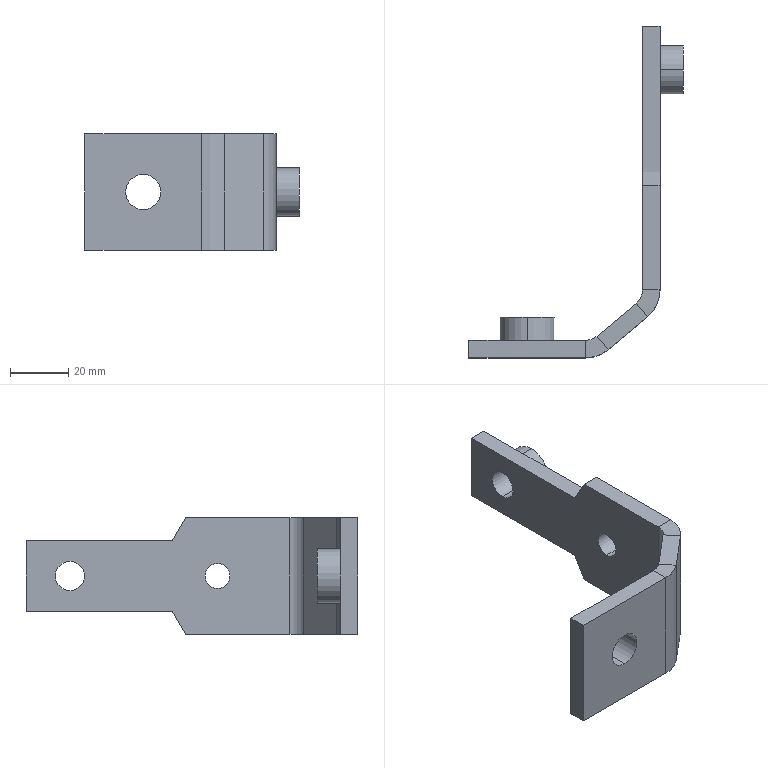Part | STEP file | 64586823 | 1 solid | 38 faces | box 73.3 x 113.5 x 40 mm | volume 34639 mm3 | plane 24 | cylinder 14 | commonest cylinder face diameters 12 x4 8.5 x2 10 x2 16.5 x2 18.5 x2 24 x2